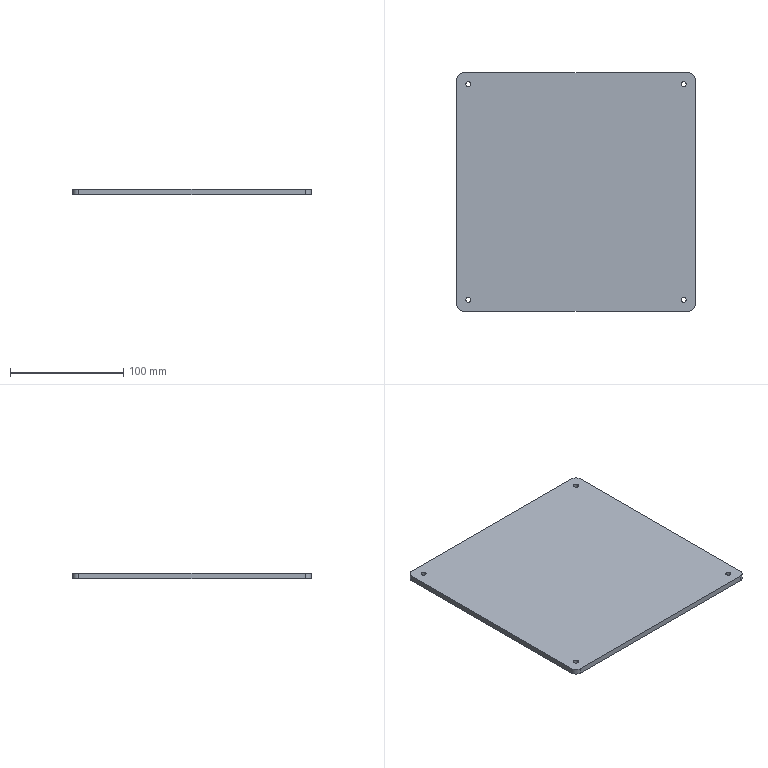Part | STEP file | Acrylic cover 2 | 1 solid | 18 faces | box 210 x 210 x 5 mm | volume 220075 mm3 | cylinder 12 | plane 6 | commonest cylinder face diameters 4.5 x8 10 x4